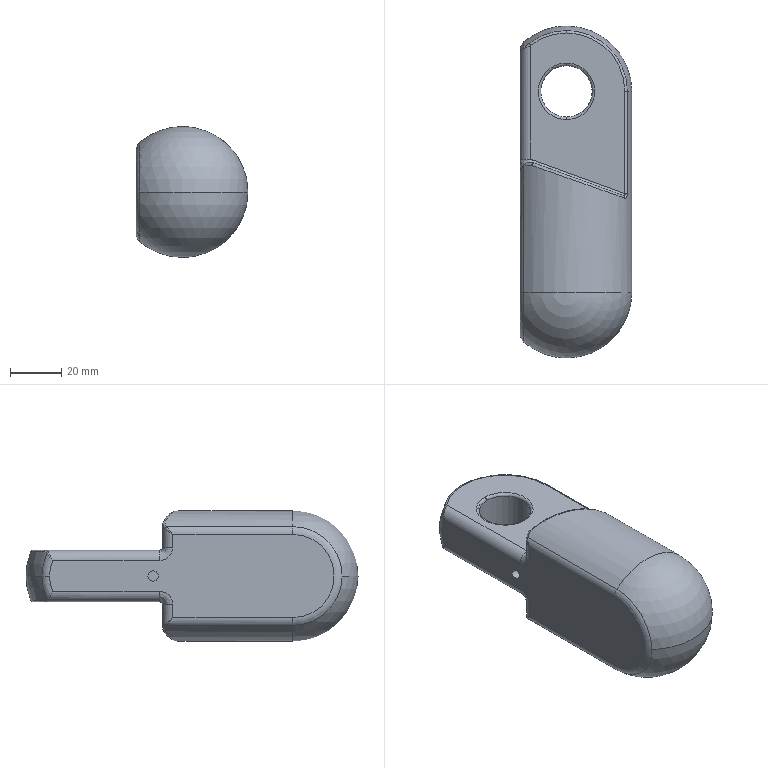Part | SolidWorks | features ICE 7, Fillet 2, MirrorPattern 1, MoveCopyBody 1, Revolution 1, Scale 1 | 1 solid | 49 faces | box 43.4 x 129 x 50.8 mm | volume 154558 mm3 | cylinder 15 | spline 14 | torus 10 | plane 6 | sphere 4 | commonest cylinder face diameters 8 x6 2 x4 4 x2 20 x2 50.8 x1